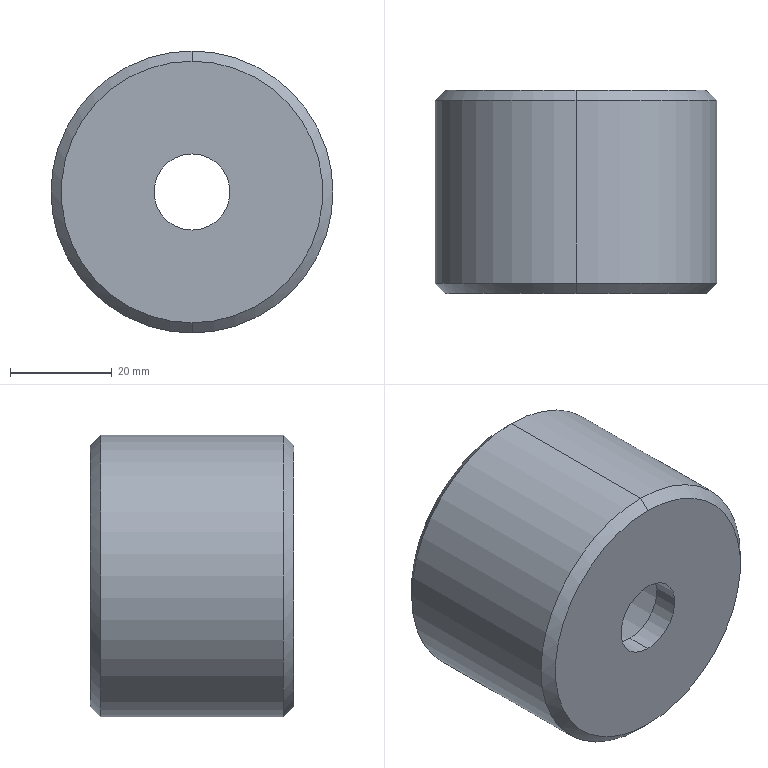Part | SolidWorks | features Chamfer 1, Extrusion 1, ICE 1 | 1 solid | 13 faces | box 55.5 x 40 x 55.5 mm | volume 67056 mm3 | cylinder 6 | cone 4 | plane 3 | commonest cylinder face diameters 15 x2 32 x2 55.5 x2
STEP:
#1=CARTESIAN_POINT('',(0.,5.,7.5));
#2=VERTEX_POINT('',#1);
#3=CARTESIAN_POINT('',(0.,5.,-7.5));
#4=VERTEX_POINT('',#3);
#5=CARTESIAN_POINT('',(0.,5.,0.));
#6=DIRECTION('',(0.,-1.,0.));
#7=DIRECTION('',(0.,0.,-1.));
#8=AXIS2_PLACEMENT_3D('',#5,#6,#7);
#9=CIRCLE('',#8,7.5);
#10=EDGE_CURVE('',#2,#4,#9,.T.);
#11=ORIENTED_EDGE('',*,*,#10,.F.);
#12=CARTESIAN_POINT('',(0.,0.,7.5));
#13=VERTEX_POINT('',#12);
#14=CARTESIAN_POINT('',(0.,5.,7.5));
#15=DIRECTION('',(0.,-1.,0.));
#16=VECTOR('',#15,1000.);
#17=LINE('',#14,#16);
#18=EDGE_CURVE('',#2,#13,#17,.T.);
#19=ORIENTED_EDGE('',*,*,#18,.T.);
#20=CARTESIAN_POINT('',(0.,0.,-7.5));
#21=VERTEX_POINT('',#20);
#22=CARTESIAN_POINT('',(0.,0.,0.));
#23=DIRECTION('',(0.,-1.,0.));
#24=DIRECTION('',(0.,0.,-1.));
#25=AXIS2_PLACEMENT_3D('',#22,#23,#24);
#26=CIRCLE('',#25,7.5);
#27=EDGE_CURVE('',#13,#21,#26,.T.);
#28=ORIENTED_EDGE('',*,*,#27,.T.);
#29=CARTESIAN_POINT('',(0.,5.,-7.5));
#30=DIRECTION('',(0.,-1.,0.));
#31=VECTOR('',#30,1000.);
#32=LINE('',#29,#31);
#33=EDGE_CURVE('',#4,#21,#32,.T.);
#34=ORIENTED_EDGE('',*,*,#33,.F.);
#35=EDGE_LOOP('',(#11,#19,#28,#34));
#36=FACE_OUTER_BOUND('',#35,.T.);
#37=CARTESIAN_POINT('',(0.,5.,0.));
#38=DIRECTION('',(0.,-1.,0.));
#39=DIRECTION('',(0.,0.,-1.));
#40=AXIS2_PLACEMENT_3D('',#37,#38,#39);
#41=CYLINDRICAL_SURFACE('',#40,7.5);
#42=ADVANCED_FACE('',(#36),#41,.F.);
#43=CARTESIAN_POINT('',(0.,0.,-25.75));
#44=VERTEX_POINT('',#43);
#45=CARTESIAN_POINT('',(0.,0.,25.75));
#46=VERTEX_POINT('',#45);
#47=CARTESIAN_POINT('',(0.,0.,0.));
#48=DIRECTION('',(0.,-1.,0.));
#49=DIRECTION('',(0.,0.,1.));
#50=AXIS2_PLACEMENT_3D('',#47,#48,#49);
#51=CIRCLE('',#50,25.75);
#52=EDGE_CURVE('',#44,#46,#51,.T.);
#53=ORIENTED_EDGE('',*,*,#52,.F.);
#54=CARTESIAN_POINT('',(0.,2.,-27.75));
#55=VERTEX_POINT('',#54);
#56=CARTESIAN_POINT('',(0.,2.,-27.75));
#57=DIRECTION('',(0.,0.7071,-0.7071));
#58=VECTOR('',#57,1000.);
#59=LINE('',#56,#58);
#60=EDGE_CURVE('',#44,#55,#59,.T.);
#61=ORIENTED_EDGE('',*,*,#60,.T.);
#62=CARTESIAN_POINT('',(0.,2.,27.75));
#63=VERTEX_POINT('',#62);
#64=CARTESIAN_POINT('',(0.,2.,0.));
#65=DIRECTION('',(0.,1.,0.));
#66=DIRECTION('',(0.,0.,1.));
#67=AXIS2_PLACEMENT_3D('',#64,#65,#66);
#68=CIRCLE('',#67,27.75);
#69=EDGE_CURVE('',#63,#55,#68,.T.);
#70=ORIENTED_EDGE('',*,*,#69,.F.);
#71=CARTESIAN_POINT('',(0.,2.,27.75));
#72=DIRECTION('',(0.,0.7071,0.7071));
#73=VECTOR('',#72,1000.);
#74=LINE('',#71,#73);
#75=EDGE_CURVE('',#46,#63,#74,.T.);
#76=ORIENTED_EDGE('',*,*,#75,.F.);
#77=EDGE_LOOP('',(#53,#61,#70,#76));
#78=FACE_OUTER_BOUND('',#77,.T.);
#79=CARTESIAN_POINT('',(0.,2.,0.));
#80=DIRECTION('',(0.,1.,0.));
#81=DIRECTION('',(0.,0.,1.));
#82=AXIS2_PLACEMENT_3D('',#79,#80,#81);
#83=CONICAL_SURFACE('',#82,27.75,0.7854);
#84=ADVANCED_FACE('',(#78),#83,.T.);
#85=CARTESIAN_POINT('',(0.,40.,25.75));
#86=VERTEX_POINT('',#85);
#87=CARTESIAN_POINT('',(0.,40.,-25.75));
#88=VERTEX_POINT('',#87);
#89=CARTESIAN_POINT('',(0.,40.,0.));
#90=DIRECTION('',(0.,1.,0.));
#91=DIRECTION('',(0.,0.,1.));
#92=AXIS2_PLACEMENT_3D('',#89,#90,#91);
#93=CIRCLE('',#92,25.75);
#94=EDGE_CURVE('',#86,#88,#93,.T.);
#95=ORIENTED_EDGE('',*,*,#94,.F.);
#96=CARTESIAN_POINT('',(0.,38.,27.75));
#97=VERTEX_POINT('',#96);
#98=CARTESIAN_POINT('',(0.,40.,25.75));
#99=DIRECTION('',(0.,-0.7071,0.7071));
#100=VECTOR('',#99,1000.);
#101=LINE('',#98,#100);
#102=EDGE_CURVE('',#86,#97,#101,.T.);
#103=ORIENTED_EDGE('',*,*,#102,.T.);
#104=CARTESIAN_POINT('',(0.,38.,-27.75));
#105=VERTEX_POINT('',#104);
#106=CARTESIAN_POINT('',(0.,38.,0.));
#107=DIRECTION('',(0.,-1.,0.));
#108=DIRECTION('',(0.,0.,1.));
#109=AXIS2_PLACEMENT_3D('',#106,#107,#108);
#110=CIRCLE('',#109,27.75);
#111=EDGE_CURVE('',#105,#97,#110,.T.);
#112=ORIENTED_EDGE('',*,*,#111,.F.);
#113=CARTESIAN_POINT('',(0.,40.,-25.75));
#114=DIRECTION('',(0.,-0.7071,-0.7071));
#115=VECTOR('',#114,1000.);
#116=LINE('',#113,#115);
#117=EDGE_CURVE('',#88,#105,#116,.T.);
#118=ORIENTED_EDGE('',*,*,#117,.F.);
#119=EDGE_LOOP('',(#95,#103,#112,#118));
#120=FACE_OUTER_BOUND('',#119,.T.);
#121=CARTESIAN_POINT('',(0.,40.,0.));
#122=DIRECTION('',(0.,-1.,0.));
#123=DIRECTION('',(0.,0.,-1.));
#124=AXIS2_PLACEMENT_3D('',#121,#122,#123);
#125=CONICAL_SURFACE('',#124,25.75,0.7854);
#126=ADVANCED_FACE('',(#120),#125,.T.);
#127=ORIENTED_EDGE('',*,*,#111,.T.);
#128=CARTESIAN_POINT('',(0.,40.,27.75));
#129=DIRECTION('',(0.,-1.,0.));
#130=VECTOR('',#129,1000.);
#131=LINE('',#128,#130);
#132=EDGE_CURVE('',#97,#63,#131,.T.);
#133=ORIENTED_EDGE('',*,*,#132,.T.);
#134=ORIENTED_EDGE('',*,*,#69,.T.);
#135=CARTESIAN_POINT('',(0.,40.,-27.75));
#136=DIRECTION('',(0.,-1.,0.));
#137=VECTOR('',#136,1000.);
#138=LINE('',#135,#137);
#139=EDGE_CURVE('',#105,#55,#138,.T.);
#140=ORIENTED_EDGE('',*,*,#139,.F.);
#141=EDGE_LOOP('',(#127,#133,#134,#140));
#142=FACE_OUTER_BOUND('',#141,.T.);
#143=CARTESIAN_POINT('',(0.,40.,0.));
#144=DIRECTION('',(0.,-1.,0.));
#145=DIRECTION('',(0.,0.,-1.));
#146=AXIS2_PLACEMENT_3D('',#143,#144,#145);
#147=CYLINDRICAL_SURFACE('',#146,27.75);
#148=ADVANCED_FACE('',(#142),#147,.T.);
#149=CARTESIAN_POINT('',(0.,40.,-16.));
#150=VERTEX_POINT('',#149);
#151=CARTESIAN_POINT('',(0.,40.,16.));
#152=VERTEX_POINT('',#151);
#153=CARTESIAN_POINT('',(0.,40.,0.));
#154=DIRECTION('',(0.,1.,0.));
#155=DIRECTION('',(0.,0.,1.));
#156=AXIS2_PLACEMENT_3D('',#153,#154,#155);
#157=CIRCLE('',#156,16.);
#158=EDGE_CURVE('',#150,#152,#157,.T.);
#159=ORIENTED_EDGE('',*,*,#158,.T.);
#160=CARTESIAN_POINT('',(0.,5.,16.));
#161=VERTEX_POINT('',#160);
#162=CARTESIAN_POINT('',(0.,40.,16.));
#163=DIRECTION('',(0.,-1.,0.));
#164=VECTOR('',#163,1000.);
#165=LINE('',#162,#164);
#166=EDGE_CURVE('',#152,#161,#165,.T.);
#167=ORIENTED_EDGE('',*,*,#166,.T.);
#168=CARTESIAN_POINT('',(0.,5.,-16.));
#169=VERTEX_POINT('',#168);
#170=CARTESIAN_POINT('',(0.,5.,0.));
#171=DIRECTION('',(0.,-1.,0.));
#172=DIRECTION('',(0.,0.,-1.));
#173=AXIS2_PLACEMENT_3D('',#170,#171,#172);
#174=CIRCLE('',#173,16.);
#175=EDGE_CURVE('',#161,#169,#174,.T.);
#176=ORIENTED_EDGE('',*,*,#175,.T.);
#177=CARTESIAN_POINT('',(0.,40.,-16.));
#178=DIRECTION('',(0.,-1.,0.));
#179=VECTOR('',#178,1000.);
#180=LINE('',#177,#179);
#181=EDGE_CURVE('',#150,#169,#180,.T.);
#182=ORIENTED_EDGE('',*,*,#181,.F.);
#183=EDGE_LOOP('',(#159,#167,#176,#182));
#184=FACE_OUTER_BOUND('',#183,.T.);
#185=CARTESIAN_POINT('',(0.,40.,0.));
#186=DIRECTION('',(0.,-1.,0.));
#187=DIRECTION('',(0.,0.,-1.));
#188=AXIS2_PLACEMENT_3D('',#185,#186,#187);
#189=CYLINDRICAL_SURFACE('',#188,16.);
#190=ADVANCED_FACE('',(#184),#189,.F.);
#191=ORIENTED_EDGE('',*,*,#166,.F.);
#192=CARTESIAN_POINT('',(0.,40.,0.));
#193=DIRECTION('',(0.,1.,0.));
#194=DIRECTION('',(0.,0.,1.));
#195=AXIS2_PLACEMENT_3D('',#192,#193,#194);
#196=CIRCLE('',#195,16.);
#197=EDGE_CURVE('',#152,#150,#196,.T.);
#198=ORIENTED_EDGE('',*,*,#197,.T.);
#199=ORIENTED_EDGE('',*,*,#181,.T.);
#200=CARTESIAN_POINT('',(0.,5.,0.));
#201=DIRECTION('',(0.,-1.,0.));
#202=DIRECTION('',(0.,0.,-1.));
#203=AXIS2_PLACEMENT_3D('',#200,#201,#202);
#204=CIRCLE('',#203,16.);
#205=EDGE_CURVE('',#169,#161,#204,.T.);
#206=ORIENTED_EDGE('',*,*,#205,.T.);
#207=EDGE_LOOP('',(#191,#198,#199,#206));
#208=FACE_OUTER_BOUND('',#207,.T.);
#209=CARTESIAN_POINT('',(0.,40.,0.));
#210=DIRECTION('',(0.,-1.,0.));
#211=DIRECTION('',(0.,0.,-1.));
#212=AXIS2_PLACEMENT_3D('',#209,#210,#211);
#213=CYLINDRICAL_SURFACE('',#212,16.);
#214=ADVANCED_FACE('',(#208),#213,.F.);
#215=CARTESIAN_POINT('',(0.,40.,0.));
#216=DIRECTION('',(0.,1.,0.));
#217=DIRECTION('',(0.,0.,1.));
#218=AXIS2_PLACEMENT_3D('',#215,#216,#217);
#219=CIRCLE('',#218,25.75);
#220=EDGE_CURVE('',#88,#86,#219,.T.);
#221=ORIENTED_EDGE('',*,*,#220,.T.);
#222=ORIENTED_EDGE('',*,*,#94,.T.);
#223=EDGE_LOOP('',(#221,#222));
#224=FACE_OUTER_BOUND('',#223,.T.);
#225=ORIENTED_EDGE('',*,*,#158,.F.);
#226=ORIENTED_EDGE('',*,*,#197,.F.);
#227=EDGE_LOOP('',(#225,#226));
#228=FACE_BOUND('',#227,.T.);
#229=CARTESIAN_POINT('',(0.,40.,0.));
#230=DIRECTION('',(0.,1.,0.));
#231=DIRECTION('',(0.,0.,1.));
#232=AXIS2_PLACEMENT_3D('',#229,#230,#231);
#233=PLANE('',#232);
#234=ADVANCED_FACE('',(#224,#228),#233,.T.);
#235=CARTESIAN_POINT('',(0.,0.,0.));
#236=DIRECTION('',(0.,-1.,0.));
#237=DIRECTION('',(0.,0.,1.));
#238=AXIS2_PLACEMENT_3D('',#235,#236,#237);
#239=CIRCLE('',#238,25.75);
#240=EDGE_CURVE('',#46,#44,#239,.T.);
#241=ORIENTED_EDGE('',*,*,#240,.T.);
#242=ORIENTED_EDGE('',*,*,#52,.T.);
#243=EDGE_LOOP('',(#241,#242));
#244=FACE_OUTER_BOUND('',#243,.T.);
#245=CARTESIAN_POINT('',(0.,0.,0.));
#246=DIRECTION('',(0.,-1.,0.));
#247=DIRECTION('',(0.,0.,-1.));
#248=AXIS2_PLACEMENT_3D('',#245,#246,#247);
#249=CIRCLE('',#248,7.5);
#250=EDGE_CURVE('',#21,#13,#249,.T.);
#251=ORIENTED_EDGE('',*,*,#250,.F.);
#252=ORIENTED_EDGE('',*,*,#27,.F.);
#253=EDGE_LOOP('',(#251,#252));
#254=FACE_BOUND('',#253,.T.);
#255=CARTESIAN_POINT('',(0.,0.,0.));
#256=DIRECTION('',(0.,1.,0.));
#257=DIRECTION('',(0.,0.,1.));
#258=AXIS2_PLACEMENT_3D('',#255,#256,#257);
#259=PLANE('',#258);
#260=ADVANCED_FACE('',(#244,#254),#259,.F.);
#261=ORIENTED_EDGE('',*,*,#132,.F.);
#262=CARTESIAN_POINT('',(0.,38.,0.));
#263=DIRECTION('',(0.,-1.,0.));
#264=DIRECTION('',(0.,0.,1.));
#265=AXIS2_PLACEMENT_3D('',#262,#263,#264);
#266=CIRCLE('',#265,27.75);
#267=EDGE_CURVE('',#97,#105,#266,.T.);
#268=ORIENTED_EDGE('',*,*,#267,.T.);
#269=ORIENTED_EDGE('',*,*,#139,.T.);
#270=CARTESIAN_POINT('',(0.,2.,0.));
#271=DIRECTION('',(0.,1.,0.));
#272=DIRECTION('',(0.,0.,1.));
#273=AXIS2_PLACEMENT_3D('',#270,#271,#272);
#274=CIRCLE('',#273,27.75);
#275=EDGE_CURVE('',#55,#63,#274,.T.);
#276=ORIENTED_EDGE('',*,*,#275,.T.);
#277=EDGE_LOOP('',(#261,#268,#269,#276));
#278=FACE_OUTER_BOUND('',#277,.T.);
#279=CARTESIAN_POINT('',(0.,40.,0.));
#280=DIRECTION('',(0.,-1.,0.));
#281=DIRECTION('',(0.,0.,-1.));
#282=AXIS2_PLACEMENT_3D('',#279,#280,#281);
#283=CYLINDRICAL_SURFACE('',#282,27.75);
#284=ADVANCED_FACE('',(#278),#283,.T.);
#285=ORIENTED_EDGE('',*,*,#102,.F.);
#286=ORIENTED_EDGE('',*,*,#220,.F.);
#287=ORIENTED_EDGE('',*,*,#117,.T.);
#288=ORIENTED_EDGE('',*,*,#267,.F.);
#289=EDGE_LOOP('',(#285,#286,#287,#288));
#290=FACE_OUTER_BOUND('',#289,.T.);
#291=CARTESIAN_POINT('',(0.,40.,0.));
#292=DIRECTION('',(0.,-1.,0.));
#293=DIRECTION('',(0.,0.,-1.));
#294=AXIS2_PLACEMENT_3D('',#291,#292,#293);
#295=CONICAL_SURFACE('',#294,25.75,0.7854);
#296=ADVANCED_FACE('',(#290),#295,.T.);
#297=ORIENTED_EDGE('',*,*,#60,.F.);
#298=ORIENTED_EDGE('',*,*,#240,.F.);
#299=ORIENTED_EDGE('',*,*,#75,.T.);
#300=ORIENTED_EDGE('',*,*,#275,.F.);
#301=EDGE_LOOP('',(#297,#298,#299,#300));
#302=FACE_OUTER_BOUND('',#301,.T.);
#303=CARTESIAN_POINT('',(0.,2.,0.));
#304=DIRECTION('',(0.,1.,0.));
#305=DIRECTION('',(0.,0.,1.));
#306=AXIS2_PLACEMENT_3D('',#303,#304,#305);
#307=CONICAL_SURFACE('',#306,27.75,0.7854);
#308=ADVANCED_FACE('',(#302),#307,.T.);
#309=CARTESIAN_POINT('',(0.,5.,0.));
#310=DIRECTION('',(0.,-1.,0.));
#311=DIRECTION('',(0.,0.,-1.));
#312=AXIS2_PLACEMENT_3D('',#309,#310,#311);
#313=CIRCLE('',#312,7.5);
#314=EDGE_CURVE('',#4,#2,#313,.T.);
#315=ORIENTED_EDGE('',*,*,#314,.T.);
#316=ORIENTED_EDGE('',*,*,#10,.T.);
#317=EDGE_LOOP('',(#315,#316));
#318=FACE_BOUND('',#317,.T.);
#319=ORIENTED_EDGE('',*,*,#205,.F.);
#320=ORIENTED_EDGE('',*,*,#175,.F.);
#321=EDGE_LOOP('',(#319,#320));
#322=FACE_OUTER_BOUND('',#321,.T.);
#323=CARTESIAN_POINT('',(0.,5.,0.));
#324=DIRECTION('',(0.,-1.,0.));
#325=DIRECTION('',(0.,0.,-1.));
#326=AXIS2_PLACEMENT_3D('',#323,#324,#325);
#327=PLANE('',#326);
#328=ADVANCED_FACE('',(#318,#322),#327,.F.);
#329=ORIENTED_EDGE('',*,*,#18,.F.);
#330=ORIENTED_EDGE('',*,*,#314,.F.);
#331=ORIENTED_EDGE('',*,*,#33,.T.);
#332=ORIENTED_EDGE('',*,*,#250,.T.);
#333=EDGE_LOOP('',(#329,#330,#331,#332));
#334=FACE_OUTER_BOUND('',#333,.T.);
#335=CARTESIAN_POINT('',(0.,5.,0.));
#336=DIRECTION('',(0.,-1.,0.));
#337=DIRECTION('',(0.,0.,-1.));
#338=AXIS2_PLACEMENT_3D('',#335,#336,#337);
#339=CYLINDRICAL_SURFACE('',#338,7.5);
#340=ADVANCED_FACE('',(#334),#339,.F.);
#341=CLOSED_SHELL('',(#42,#84,#126,#148,#190,#214,#234,#260,#284,#296,#308,#328,#340));
#342=MANIFOLD_SOLID_BREP('',#341);
#343=CARTESIAN_POINT('',(0.,0.,0.));
#344=DIRECTION('',(0.,0.,1.));
#345=DIRECTION('',(1.,0.,0.));
#346=AXIS2_PLACEMENT_3D('',#343,#344,#345);
#347=(LENGTH_UNIT()NAMED_UNIT(*)SI_UNIT(.MILLI.,.METRE.));
#348=UNCERTAINTY_MEASURE_WITH_UNIT(LENGTH_MEASURE(0.00001),#347,'','');
#349=(NAMED_UNIT(*)PLANE_ANGLE_UNIT()SI_UNIT($,.RADIAN.));
#350=(NAMED_UNIT(*)SI_UNIT($,.STERADIAN.)SOLID_ANGLE_UNIT());
#351=(GEOMETRIC_REPRESENTATION_CONTEXT(3)GLOBAL_UNCERTAINTY_ASSIGNED_CONTEXT((#348))GLOBAL_UNIT_ASSIGNED_CONTEXT((#347,#349,#350))REPRESENTATION_CONTEXT('',''));
#352=ADVANCED_BREP_SHAPE_REPRESENTATION('',(#342,#346),#351);